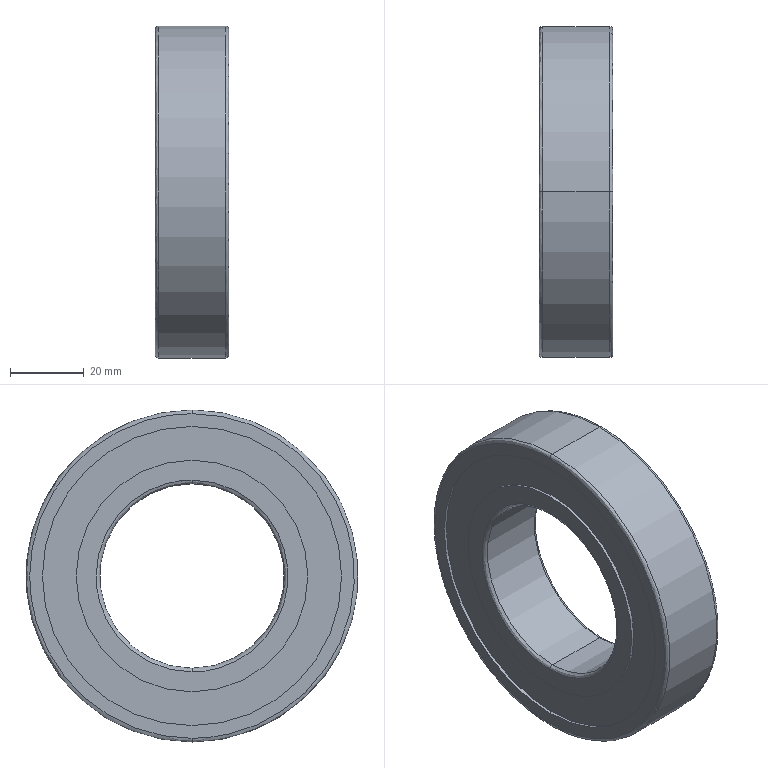Part | STEP file | B6210ZZ | 1 solid | 26 faces | box 20 x 90 x 90 mm | volume 84481 mm3 | cylinder 12 | spline 8 | plane 6 | commonest cylinder face diameters 62.8 x4 81.06 x4 50 x2 90 x2